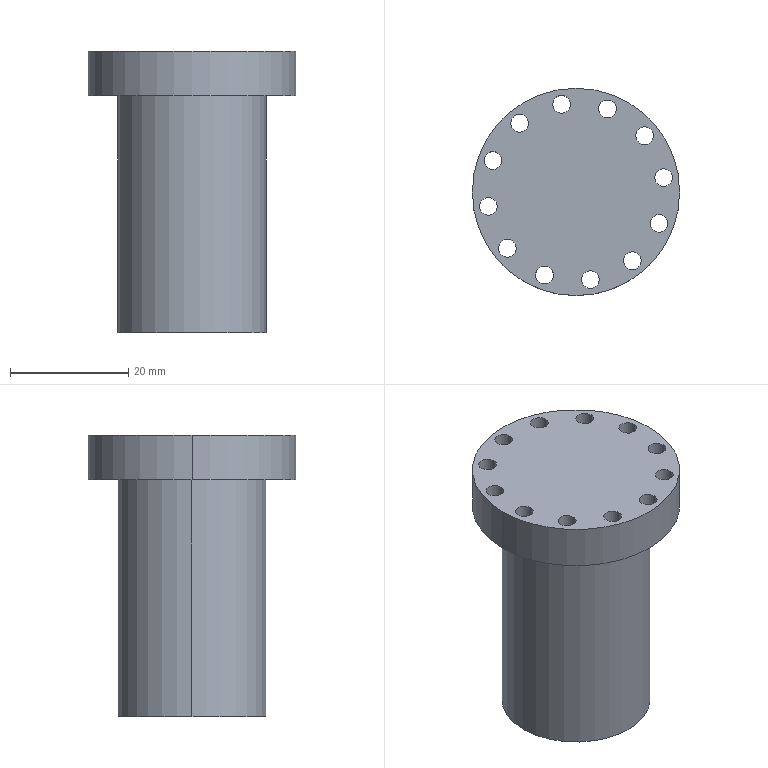Part | SolidWorks | features Cut 1, Extrusion 1, ICE 1 | 1 solid | 31 faces | box 35 x 35 x 47.5 mm | volume 26215 mm3 | cylinder 28 | plane 3 | commonest cylinder face diameters 3 x24 25 x2 35 x2
STEP:
#1=CARTESIAN_POINT('',(-76.803,10.969,0.));
#2=VERTEX_POINT('',#1);
#3=CARTESIAN_POINT('',(-73.803,10.969,0.));
#4=VERTEX_POINT('',#3);
#5=CARTESIAN_POINT('',(-75.303,10.969,0.));
#6=DIRECTION('',(0.,0.,1.));
#7=DIRECTION('',(1.,0.,0.));
#8=AXIS2_PLACEMENT_3D('',#5,#6,#7);
#9=CIRCLE('',#8,1.5);
#10=EDGE_CURVE('',#2,#4,#9,.T.);
#11=ORIENTED_EDGE('',*,*,#10,.F.);
#12=CARTESIAN_POINT('',(-76.803,10.969,7.5));
#13=VERTEX_POINT('',#12);
#14=CARTESIAN_POINT('',(-76.803,10.969,-40.));
#15=DIRECTION('',(0.,0.,1.));
#16=VECTOR('',#15,1000.);
#17=LINE('',#14,#16);
#18=EDGE_CURVE('',#2,#13,#17,.T.);
#19=ORIENTED_EDGE('',*,*,#18,.T.);
#20=CARTESIAN_POINT('',(-73.803,10.969,7.5));
#21=VERTEX_POINT('',#20);
#22=CARTESIAN_POINT('',(-75.303,10.969,7.5));
#23=DIRECTION('',(0.,0.,1.));
#24=DIRECTION('',(1.,0.,0.));
#25=AXIS2_PLACEMENT_3D('',#22,#23,#24);
#26=CIRCLE('',#25,1.5);
#27=EDGE_CURVE('',#13,#21,#26,.T.);
#28=ORIENTED_EDGE('',*,*,#27,.T.);
#29=CARTESIAN_POINT('',(-73.803,10.969,-40.));
#30=DIRECTION('',(0.,0.,1.));
#31=VECTOR('',#30,1000.);
#32=LINE('',#29,#31);
#33=EDGE_CURVE('',#4,#21,#32,.T.);
#34=ORIENTED_EDGE('',*,*,#33,.F.);
#35=EDGE_LOOP('',(#11,#19,#28,#34));
#36=FACE_OUTER_BOUND('',#35,.T.);
#37=CARTESIAN_POINT('',(-75.303,10.969,-40.));
#38=DIRECTION('',(0.,0.,1.));
#39=DIRECTION('',(1.,0.,0.));
#40=AXIS2_PLACEMENT_3D('',#37,#38,#39);
#41=CYLINDRICAL_SURFACE('',#40,1.5);
#42=ADVANCED_FACE('',(#36),#41,.F.);
#43=CARTESIAN_POINT('',(-69.077,10.197,0.));
#44=VERTEX_POINT('',#43);
#45=CARTESIAN_POINT('',(-66.077,10.197,0.));
#46=VERTEX_POINT('',#45);
#47=CARTESIAN_POINT('',(-67.577,10.197,0.));
#48=DIRECTION('',(0.,0.,1.));
#49=DIRECTION('',(1.,0.,0.));
#50=AXIS2_PLACEMENT_3D('',#47,#48,#49);
#51=CIRCLE('',#50,1.5);
#52=EDGE_CURVE('',#44,#46,#51,.T.);
#53=ORIENTED_EDGE('',*,*,#52,.F.);
#54=CARTESIAN_POINT('',(-69.077,10.197,7.5));
#55=VERTEX_POINT('',#54);
#56=CARTESIAN_POINT('',(-69.077,10.197,-40.));
#57=DIRECTION('',(0.,0.,1.));
#58=VECTOR('',#57,1000.);
#59=LINE('',#56,#58);
#60=EDGE_CURVE('',#44,#55,#59,.T.);
#61=ORIENTED_EDGE('',*,*,#60,.T.);
#62=CARTESIAN_POINT('',(-66.077,10.197,7.5));
#63=VERTEX_POINT('',#62);
#64=CARTESIAN_POINT('',(-67.577,10.197,7.5));
#65=DIRECTION('',(0.,0.,1.));
#66=DIRECTION('',(1.,0.,0.));
#67=AXIS2_PLACEMENT_3D('',#64,#65,#66);
#68=CIRCLE('',#67,1.5);
#69=EDGE_CURVE('',#55,#63,#68,.T.);
#70=ORIENTED_EDGE('',*,*,#69,.T.);
#71=CARTESIAN_POINT('',(-66.077,10.197,-40.));
#72=DIRECTION('',(0.,0.,1.));
#73=VECTOR('',#72,1000.);
#74=LINE('',#71,#73);
#75=EDGE_CURVE('',#46,#63,#74,.T.);
#76=ORIENTED_EDGE('',*,*,#75,.F.);
#77=EDGE_LOOP('',(#53,#61,#70,#76));
#78=FACE_OUTER_BOUND('',#77,.T.);
#79=CARTESIAN_POINT('',(-67.577,10.197,-40.));
#80=DIRECTION('',(0.,0.,1.));
#81=DIRECTION('',(1.,0.,0.));
#82=AXIS2_PLACEMENT_3D('',#79,#80,#81);
#83=CYLINDRICAL_SURFACE('',#82,1.5);
#84=ADVANCED_FACE('',(#78),#83,.F.);
#85=CARTESIAN_POINT('',(-62.,13.392,0.));
#86=VERTEX_POINT('',#85);
#87=CARTESIAN_POINT('',(-59.,13.392,0.));
#88=VERTEX_POINT('',#87);
#89=CARTESIAN_POINT('',(-60.5,13.392,0.));
#90=DIRECTION('',(0.,0.,1.));
#91=DIRECTION('',(1.,0.,0.));
#92=AXIS2_PLACEMENT_3D('',#89,#90,#91);
#93=CIRCLE('',#92,1.5);
#94=EDGE_CURVE('',#86,#88,#93,.T.);
#95=ORIENTED_EDGE('',*,*,#94,.F.);
#96=CARTESIAN_POINT('',(-62.,13.392,7.5));
#97=VERTEX_POINT('',#96);
#98=CARTESIAN_POINT('',(-62.,13.392,-40.));
#99=DIRECTION('',(0.,0.,1.));
#100=VECTOR('',#99,1000.);
#101=LINE('',#98,#100);
#102=EDGE_CURVE('',#86,#97,#101,.T.);
#103=ORIENTED_EDGE('',*,*,#102,.T.);
#104=CARTESIAN_POINT('',(-59.,13.392,7.5));
#105=VERTEX_POINT('',#104);
#106=CARTESIAN_POINT('',(-60.5,13.392,7.5));
#107=DIRECTION('',(0.,0.,1.));
#108=DIRECTION('',(1.,0.,0.));
#109=AXIS2_PLACEMENT_3D('',#106,#107,#108);
#110=CIRCLE('',#109,1.5);
#111=EDGE_CURVE('',#97,#105,#110,.T.);
#112=ORIENTED_EDGE('',*,*,#111,.T.);
#113=CARTESIAN_POINT('',(-59.,13.392,-40.));
#114=DIRECTION('',(0.,0.,1.));
#115=VECTOR('',#114,1000.);
#116=LINE('',#113,#115);
#117=EDGE_CURVE('',#88,#105,#116,.T.);
#118=ORIENTED_EDGE('',*,*,#117,.F.);
#119=EDGE_LOOP('',(#95,#103,#112,#118));
#120=FACE_OUTER_BOUND('',#119,.T.);
#121=CARTESIAN_POINT('',(-60.5,13.392,-40.));
#122=DIRECTION('',(0.,0.,1.));
#123=DIRECTION('',(1.,0.,0.));
#124=AXIS2_PLACEMENT_3D('',#121,#122,#123);
#125=CYLINDRICAL_SURFACE('',#124,1.5);
#126=ADVANCED_FACE('',(#120),#125,.F.);
#127=CARTESIAN_POINT('',(-57.469,19.697,0.));
#128=VERTEX_POINT('',#127);
#129=CARTESIAN_POINT('',(-54.469,19.697,0.));
#130=VERTEX_POINT('',#129);
#131=CARTESIAN_POINT('',(-55.969,19.697,0.));
#132=DIRECTION('',(0.,0.,1.));
#133=DIRECTION('',(1.,0.,0.));
#134=AXIS2_PLACEMENT_3D('',#131,#132,#133);
#135=CIRCLE('',#134,1.5);
#136=EDGE_CURVE('',#128,#130,#135,.T.);
#137=ORIENTED_EDGE('',*,*,#136,.F.);
#138=CARTESIAN_POINT('',(-57.469,19.697,7.5));
#139=VERTEX_POINT('',#138);
#140=CARTESIAN_POINT('',(-57.469,19.697,-40.));
#141=DIRECTION('',(0.,0.,1.));
#142=VECTOR('',#141,1000.);
#143=LINE('',#140,#142);
#144=EDGE_CURVE('',#128,#139,#143,.T.);
#145=ORIENTED_EDGE('',*,*,#144,.T.);
#146=CARTESIAN_POINT('',(-54.469,19.697,7.5));
#147=VERTEX_POINT('',#146);
#148=CARTESIAN_POINT('',(-55.969,19.697,7.5));
#149=DIRECTION('',(0.,0.,1.));
#150=DIRECTION('',(1.,0.,0.));
#151=AXIS2_PLACEMENT_3D('',#148,#149,#150);
#152=CIRCLE('',#151,1.5);
#153=EDGE_CURVE('',#139,#147,#152,.T.);
#154=ORIENTED_EDGE('',*,*,#153,.T.);
#155=CARTESIAN_POINT('',(-54.469,19.697,-40.));
#156=DIRECTION('',(0.,0.,1.));
#157=VECTOR('',#156,1000.);
#158=LINE('',#155,#157);
#159=EDGE_CURVE('',#130,#147,#158,.T.);
#160=ORIENTED_EDGE('',*,*,#159,.F.);
#161=EDGE_LOOP('',(#137,#145,#154,#160));
#162=FACE_OUTER_BOUND('',#161,.T.);
#163=CARTESIAN_POINT('',(-55.969,19.697,-40.));
#164=DIRECTION('',(0.,0.,1.));
#165=DIRECTION('',(1.,0.,0.));
#166=AXIS2_PLACEMENT_3D('',#163,#164,#165);
#167=CYLINDRICAL_SURFACE('',#166,1.5);
#168=ADVANCED_FACE('',(#162),#167,.F.);
#169=CARTESIAN_POINT('',(-56.697,27.423,0.));
#170=VERTEX_POINT('',#169);
#171=CARTESIAN_POINT('',(-53.697,27.423,0.));
#172=VERTEX_POINT('',#171);
#173=CARTESIAN_POINT('',(-55.197,27.423,0.));
#174=DIRECTION('',(0.,0.,1.));
#175=DIRECTION('',(1.,0.,0.));
#176=AXIS2_PLACEMENT_3D('',#173,#174,#175);
#177=CIRCLE('',#176,1.5);
#178=EDGE_CURVE('',#170,#172,#177,.T.);
#179=ORIENTED_EDGE('',*,*,#178,.F.);
#180=CARTESIAN_POINT('',(-56.697,27.423,7.5));
#181=VERTEX_POINT('',#180);
#182=CARTESIAN_POINT('',(-56.697,27.423,-40.));
#183=DIRECTION('',(0.,0.,1.));
#184=VECTOR('',#183,1000.);
#185=LINE('',#182,#184);
#186=EDGE_CURVE('',#170,#181,#185,.T.);
#187=ORIENTED_EDGE('',*,*,#186,.T.);
#188=CARTESIAN_POINT('',(-53.697,27.423,7.5));
#189=VERTEX_POINT('',#188);
#190=CARTESIAN_POINT('',(-55.197,27.423,7.5));
#191=DIRECTION('',(0.,0.,1.));
#192=DIRECTION('',(1.,0.,0.));
#193=AXIS2_PLACEMENT_3D('',#190,#191,#192);
#194=CIRCLE('',#193,1.5);
#195=EDGE_CURVE('',#181,#189,#194,.T.);
#196=ORIENTED_EDGE('',*,*,#195,.T.);
#197=CARTESIAN_POINT('',(-53.697,27.423,-40.));
#198=DIRECTION('',(0.,0.,1.));
#199=VECTOR('',#198,1000.);
#200=LINE('',#197,#199);
#201=EDGE_CURVE('',#172,#189,#200,.T.);
#202=ORIENTED_EDGE('',*,*,#201,.F.);
#203=EDGE_LOOP('',(#179,#187,#196,#202));
#204=FACE_OUTER_BOUND('',#203,.T.);
#205=CARTESIAN_POINT('',(-55.197,27.423,-40.));
#206=DIRECTION('',(0.,0.,1.));
#207=DIRECTION('',(1.,0.,0.));
#208=AXIS2_PLACEMENT_3D('',#205,#206,#207);
#209=CYLINDRICAL_SURFACE('',#208,1.5);
#210=ADVANCED_FACE('',(#204),#209,.F.);
#211=CARTESIAN_POINT('',(-59.892,34.5,0.));
#212=VERTEX_POINT('',#211);
#213=CARTESIAN_POINT('',(-56.892,34.5,0.));
#214=VERTEX_POINT('',#213);
#215=CARTESIAN_POINT('',(-58.392,34.5,0.));
#216=DIRECTION('',(0.,0.,1.));
#217=DIRECTION('',(1.,0.,0.));
#218=AXIS2_PLACEMENT_3D('',#215,#216,#217);
#219=CIRCLE('',#218,1.5);
#220=EDGE_CURVE('',#212,#214,#219,.T.);
#221=ORIENTED_EDGE('',*,*,#220,.F.);
#222=CARTESIAN_POINT('',(-59.892,34.5,7.5));
#223=VERTEX_POINT('',#222);
#224=CARTESIAN_POINT('',(-59.892,34.5,-40.));
#225=DIRECTION('',(0.,0.,1.));
#226=VECTOR('',#225,1000.);
#227=LINE('',#224,#226);
#228=EDGE_CURVE('',#212,#223,#227,.T.);
#229=ORIENTED_EDGE('',*,*,#228,.T.);
#230=CARTESIAN_POINT('',(-56.892,34.5,7.5));
#231=VERTEX_POINT('',#230);
#232=CARTESIAN_POINT('',(-58.392,34.5,7.5));
#233=DIRECTION('',(0.,0.,1.));
#234=DIRECTION('',(1.,0.,0.));
#235=AXIS2_PLACEMENT_3D('',#232,#233,#234);
#236=CIRCLE('',#235,1.5);
#237=EDGE_CURVE('',#223,#231,#236,.T.);
#238=ORIENTED_EDGE('',*,*,#237,.T.);
#239=CARTESIAN_POINT('',(-56.892,34.5,-40.));
#240=DIRECTION('',(0.,0.,1.));
#241=VECTOR('',#240,1000.);
#242=LINE('',#239,#241);
#243=EDGE_CURVE('',#214,#231,#242,.T.);
#244=ORIENTED_EDGE('',*,*,#243,.F.);
#245=EDGE_LOOP('',(#221,#229,#238,#244));
#246=FACE_OUTER_BOUND('',#245,.T.);
#247=CARTESIAN_POINT('',(-58.392,34.5,-40.));
#248=DIRECTION('',(0.,0.,1.));
#249=DIRECTION('',(1.,0.,0.));
#250=AXIS2_PLACEMENT_3D('',#247,#248,#249);
#251=CYLINDRICAL_SURFACE('',#250,1.5);
#252=ADVANCED_FACE('',(#246),#251,.F.);
#253=CARTESIAN_POINT('',(-66.197,39.031,0.));
#254=VERTEX_POINT('',#253);
#255=CARTESIAN_POINT('',(-63.197,39.031,0.));
#256=VERTEX_POINT('',#255);
#257=CARTESIAN_POINT('',(-64.697,39.031,0.));
#258=DIRECTION('',(0.,0.,1.));
#259=DIRECTION('',(1.,0.,0.));
#260=AXIS2_PLACEMENT_3D('',#257,#258,#259);
#261=CIRCLE('',#260,1.5);
#262=EDGE_CURVE('',#254,#256,#261,.T.);
#263=ORIENTED_EDGE('',*,*,#262,.F.);
#264=CARTESIAN_POINT('',(-66.197,39.031,7.5));
#265=VERTEX_POINT('',#264);
#266=CARTESIAN_POINT('',(-66.197,39.031,-40.));
#267=DIRECTION('',(0.,0.,1.));
#268=VECTOR('',#267,1000.);
#269=LINE('',#266,#268);
#270=EDGE_CURVE('',#254,#265,#269,.T.);
#271=ORIENTED_EDGE('',*,*,#270,.T.);
#272=CARTESIAN_POINT('',(-63.197,39.031,7.5));
#273=VERTEX_POINT('',#272);
#274=CARTESIAN_POINT('',(-64.697,39.031,7.5));
#275=DIRECTION('',(0.,0.,1.));
#276=DIRECTION('',(1.,0.,0.));
#277=AXIS2_PLACEMENT_3D('',#274,#275,#276);
#278=CIRCLE('',#277,1.5);
#279=EDGE_CURVE('',#265,#273,#278,.T.);
#280=ORIENTED_EDGE('',*,*,#279,.T.);
#281=CARTESIAN_POINT('',(-63.197,39.031,-40.));
#282=DIRECTION('',(0.,0.,1.));
#283=VECTOR('',#282,1000.);
#284=LINE('',#281,#283);
#285=EDGE_CURVE('',#256,#273,#284,.T.);
#286=ORIENTED_EDGE('',*,*,#285,.F.);
#287=EDGE_LOOP('',(#263,#271,#280,#286));
#288=FACE_OUTER_BOUND('',#287,.T.);
#289=CARTESIAN_POINT('',(-64.697,39.031,-40.));
#290=DIRECTION('',(0.,0.,1.));
#291=DIRECTION('',(1.,0.,0.));
#292=AXIS2_PLACEMENT_3D('',#289,#290,#291);
#293=CYLINDRICAL_SURFACE('',#292,1.5);
#294=ADVANCED_FACE('',(#288),#293,.F.);
#295=CARTESIAN_POINT('',(-73.923,39.803,0.));
#296=VERTEX_POINT('',#295);
#297=CARTESIAN_POINT('',(-70.923,39.803,0.));
#298=VERTEX_POINT('',#297);
#299=CARTESIAN_POINT('',(-72.423,39.803,0.));
#300=DIRECTION('',(0.,0.,1.));
#301=DIRECTION('',(1.,0.,0.));
#302=AXIS2_PLACEMENT_3D('',#299,#300,#301);
#303=CIRCLE('',#302,1.5);
#304=EDGE_CURVE('',#296,#298,#303,.T.);
#305=ORIENTED_EDGE('',*,*,#304,.F.);
#306=CARTESIAN_POINT('',(-73.923,39.803,7.5));
#307=VERTEX_POINT('',#306);
#308=CARTESIAN_POINT('',(-73.923,39.803,-40.));
#309=DIRECTION('',(0.,0.,1.));
#310=VECTOR('',#309,1000.);
#311=LINE('',#308,#310);
#312=EDGE_CURVE('',#296,#307,#311,.T.);
#313=ORIENTED_EDGE('',*,*,#312,.T.);
#314=CARTESIAN_POINT('',(-70.923,39.803,7.5));
#315=VERTEX_POINT('',#314);
#316=CARTESIAN_POINT('',(-72.423,39.803,7.5));
#317=DIRECTION('',(0.,0.,1.));
#318=DIRECTION('',(1.,0.,0.));
#319=AXIS2_PLACEMENT_3D('',#316,#317,#318);
#320=CIRCLE('',#319,1.5);
#321=EDGE_CURVE('',#307,#315,#320,.T.);
#322=ORIENTED_EDGE('',*,*,#321,.T.);
#323=CARTESIAN_POINT('',(-70.923,39.803,-40.));
#324=DIRECTION('',(0.,0.,1.));
#325=VECTOR('',#324,1000.);
#326=LINE('',#323,#325);
#327=EDGE_CURVE('',#298,#315,#326,.T.);
#328=ORIENTED_EDGE('',*,*,#327,.F.);
#329=EDGE_LOOP('',(#305,#313,#322,#328));
#330=FACE_OUTER_BOUND('',#329,.T.);
#331=CARTESIAN_POINT('',(-72.423,39.803,-40.));
#332=DIRECTION('',(0.,0.,1.));
#333=DIRECTION('',(1.,0.,0.));
#334=AXIS2_PLACEMENT_3D('',#331,#332,#333);
#335=CYLINDRICAL_SURFACE('',#334,1.5);
#336=ADVANCED_FACE('',(#330),#335,.F.);
#337=CARTESIAN_POINT('',(-81.,36.608,0.));
#338=VERTEX_POINT('',#337);
#339=CARTESIAN_POINT('',(-78.,36.608,0.));
#340=VERTEX_POINT('',#339);
#341=CARTESIAN_POINT('',(-79.5,36.608,0.));
#342=DIRECTION('',(0.,0.,1.));
#343=DIRECTION('',(1.,0.,0.));
#344=AXIS2_PLACEMENT_3D('',#341,#342,#343);
#345=CIRCLE('',#344,1.5);
#346=EDGE_CURVE('',#338,#340,#345,.T.);
#347=ORIENTED_EDGE('',*,*,#346,.F.);
#348=CARTESIAN_POINT('',(-81.,36.608,7.5));
#349=VERTEX_POINT('',#348);
#350=CARTESIAN_POINT('',(-81.,36.608,-40.));
#351=DIRECTION('',(0.,0.,1.));
#352=VECTOR('',#351,1000.);
#353=LINE('',#350,#352);
#354=EDGE_CURVE('',#338,#349,#353,.T.);
#355=ORIENTED_EDGE('',*,*,#354,.T.);
#356=CARTESIAN_POINT('',(-78.,36.608,7.5));
#357=VERTEX_POINT('',#356);
#358=CARTESIAN_POINT('',(-79.5,36.608,7.5));
#359=DIRECTION('',(0.,0.,1.));
#360=DIRECTION('',(1.,0.,0.));
#361=AXIS2_PLACEMENT_3D('',#358,#359,#360);
#362=CIRCLE('',#361,1.5);
#363=EDGE_CURVE('',#349,#357,#362,.T.);
#364=ORIENTED_EDGE('',*,*,#363,.T.);
#365=CARTESIAN_POINT('',(-78.,36.608,-40.));
#366=DIRECTION('',(0.,0.,1.));
#367=VECTOR('',#366,1000.);
#368=LINE('',#365,#367);
#369=EDGE_CURVE('',#340,#357,#368,.T.);
#370=ORIENTED_EDGE('',*,*,#369,.F.);
#371=EDGE_LOOP('',(#347,#355,#364,#370));
#372=FACE_OUTER_BOUND('',#371,.T.);
#373=CARTESIAN_POINT('',(-79.5,36.608,-40.));
#374=DIRECTION('',(0.,0.,1.));
#375=DIRECTION('',(1.,0.,0.));
#376=AXIS2_PLACEMENT_3D('',#373,#374,#375);
#377=CYLINDRICAL_SURFACE('',#376,1.5);
#378=ADVANCED_FACE('',(#372),#377,.F.);
#379=CARTESIAN_POINT('',(-85.531,30.303,0.));
#380=VERTEX_POINT('',#379);
#381=CARTESIAN_POINT('',(-82.531,30.303,0.));
#382=VERTEX_POINT('',#381);
#383=CARTESIAN_POINT('',(-84.031,30.303,0.));
#384=DIRECTION('',(0.,0.,1.));
#385=DIRECTION('',(1.,0.,0.));
#386=AXIS2_PLACEMENT_3D('',#383,#384,#385);
#387=CIRCLE('',#386,1.5);
#388=EDGE_CURVE('',#380,#382,#387,.T.);
#389=ORIENTED_EDGE('',*,*,#388,.F.);
#390=CARTESIAN_POINT('',(-85.531,30.303,7.5));
#391=VERTEX_POINT('',#390);
#392=CARTESIAN_POINT('',(-85.531,30.303,-40.));
#393=DIRECTION('',(0.,0.,1.));
#394=VECTOR('',#393,1000.);
#395=LINE('',#392,#394);
#396=EDGE_CURVE('',#380,#391,#395,.T.);
#397=ORIENTED_EDGE('',*,*,#396,.T.);
#398=CARTESIAN_POINT('',(-82.531,30.303,7.5));
#399=VERTEX_POINT('',#398);
#400=CARTESIAN_POINT('',(-84.031,30.303,7.5));
#401=DIRECTION('',(0.,0.,1.));
#402=DIRECTION('',(1.,0.,0.));
#403=AXIS2_PLACEMENT_3D('',#400,#401,#402);
#404=CIRCLE('',#403,1.5);
#405=EDGE_CURVE('',#391,#399,#404,.T.);
#406=ORIENTED_EDGE('',*,*,#405,.T.);
#407=CARTESIAN_POINT('',(-82.531,30.303,-40.));
#408=DIRECTION('',(0.,0.,1.));
#409=VECTOR('',#408,1000.);
#410=LINE('',#407,#409);
#411=EDGE_CURVE('',#382,#399,#410,.T.);
#412=ORIENTED_EDGE('',*,*,#411,.F.);
#413=EDGE_LOOP('',(#389,#397,#406,#412));
#414=FACE_OUTER_BOUND('',#413,.T.);
#415=CARTESIAN_POINT('',(-84.031,30.303,-40.));
#416=DIRECTION('',(0.,0.,1.));
#417=DIRECTION('',(1.,0.,0.));
#418=AXIS2_PLACEMENT_3D('',#415,#416,#417);
#419=CYLINDRICAL_SURFACE('',#418,1.5);
#420=ADVANCED_FACE('',(#414),#419,.F.);
#421=CARTESIAN_POINT('',(-86.303,22.577,0.));
#422=VERTEX_POINT('',#421);
#423=CARTESIAN_POINT('',(-83.303,22.577,0.));
#424=VERTEX_POINT('',#423);
#425=CARTESIAN_POINT('',(-84.803,22.577,0.));
#426=DIRECTION('',(0.,0.,1.));
#427=DIRECTION('',(1.,0.,0.));
#428=AXIS2_PLACEMENT_3D('',#425,#426,#427);
#429=CIRCLE('',#428,1.5);
#430=EDGE_CURVE('',#422,#424,#429,.T.);
#431=ORIENTED_EDGE('',*,*,#430,.F.);
#432=CARTESIAN_POINT('',(-86.303,22.577,7.5));
#433=VERTEX_POINT('',#432);
#434=CARTESIAN_POINT('',(-86.303,22.577,-40.));
#435=DIRECTION('',(0.,0.,1.));
#436=VECTOR('',#435,1000.);
#437=LINE('',#434,#436);
#438=EDGE_CURVE('',#422,#433,#437,.T.);
#439=ORIENTED_EDGE('',*,*,#438,.T.);
#440=CARTESIAN_POINT('',(-83.303,22.577,7.5));
#441=VERTEX_POINT('',#440);
#442=CARTESIAN_POINT('',(-84.803,22.577,7.5));
#443=DIRECTION('',(0.,0.,1.));
#444=DIRECTION('',(1.,0.,0.));
#445=AXIS2_PLACEMENT_3D('',#442,#443,#444);
#446=CIRCLE('',#445,1.5);
#447=EDGE_CURVE('',#433,#441,#446,.T.);
#448=ORIENTED_EDGE('',*,*,#447,.T.);
#449=CARTESIAN_POINT('',(-83.303,22.577,-40.));
#450=DIRECTION('',(0.,0.,1.));
#451=VECTOR('',#450,1000.);
#452=LINE('',#449,#451);
#453=EDGE_CURVE('',#424,#441,#452,.T.);
#454=ORIENTED_EDGE('',*,*,#453,.F.);
#455=EDGE_LOOP('',(#431,#439,#448,#454));
#456=FACE_OUTER_BOUND('',#455,.T.);
#457=CARTESIAN_POINT('',(-84.803,22.577,-40.));
#458=DIRECTION('',(0.,0.,1.));
#459=DIRECTION('',(1.,0.,0.));
#460=AXIS2_PLACEMENT_3D('',#457,#458,#459);
#461=CYLINDRICAL_SURFACE('',#460,1.5);
#462=ADVANCED_FACE('',(#456),#461,.F.);
#463=CARTESIAN_POINT('',(-83.108,15.5,0.));
#464=VERTEX_POINT('',#463);
#465=CARTESIAN_POINT('',(-80.108,15.5,0.));
#466=VERTEX_POINT('',#465);
#467=CARTESIAN_POINT('',(-81.608,15.5,0.));
#468=DIRECTION('',(0.,0.,1.));
#469=DIRECTION('',(1.,0.,0.));
#470=AXIS2_PLACEMENT_3D('',#467,#468,#469);
#471=CIRCLE('',#470,1.5);
#472=EDGE_CURVE('',#464,#466,#471,.T.);
#473=ORIENTED_EDGE('',*,*,#472,.F.);
#474=CARTESIAN_POINT('',(-83.108,15.5,7.5));
#475=VERTEX_POINT('',#474);
#476=CARTESIAN_POINT('',(-83.108,15.5,-40.));
#477=DIRECTION('',(0.,0.,1.));
#478=VECTOR('',#477,1000.);
#479=LINE('',#476,#478);
#480=EDGE_CURVE('',#464,#475,#479,.T.);
#481=ORIENTED_EDGE('',*,*,#480,.T.);
#482=CARTESIAN_POINT('',(-80.108,15.5,7.5));
#483=VERTEX_POINT('',#482);
#484=CARTESIAN_POINT('',(-81.608,15.5,7.5));
#485=DIRECTION('',(0.,0.,1.));
#486=DIRECTION('',(1.,0.,0.));
#487=AXIS2_PLACEMENT_3D('',#484,#485,#486);
#488=CIRCLE('',#487,1.5);
#489=EDGE_CURVE('',#475,#483,#488,.T.);
#490=ORIENTED_EDGE('',*,*,#489,.T.);
#491=CARTESIAN_POINT('',(-80.108,15.5,-40.));
#492=DIRECTION('',(0.,0.,1.));
#493=VECTOR('',#492,1000.);
#494=LINE('',#491,#493);
#495=EDGE_CURVE('',#466,#483,#494,.T.);
#496=ORIENTED_EDGE('',*,*,#495,.F.);
#497=EDGE_LOOP('',(#473,#481,#490,#496));
#498=FACE_OUTER_BOUND('',#497,.T.);
#499=CARTESIAN_POINT('',(-81.608,15.5,-40.));
#500=DIRECTION('',(0.,0.,1.));
#501=DIRECTION('',(1.,0.,0.));
#502=AXIS2_PLACEMENT_3D('',#499,#500,#501);
#503=CYLINDRICAL_SURFACE('',#502,1.5);
#504=ADVANCED_FACE('',(#498),#503,.F.);
#505=CARTESIAN_POINT('',(-82.5,25.,-40.));
#506=VERTEX_POINT('',#505);
#507=CARTESIAN_POINT('',(-57.5,25.,-40.));
#508=VERTEX_POINT('',#507);
#509=CARTESIAN_POINT('',(-70.,25.,-40.));
#510=DIRECTION('',(0.,0.,-1.));
#511=DIRECTION('',(-1.,0.,0.));
#512=AXIS2_PLACEMENT_3D('',#509,#510,#511);
#513=CIRCLE('',#512,12.5);
#514=EDGE_CURVE('',#506,#508,#513,.T.);
#515=ORIENTED_EDGE('',*,*,#514,.F.);
#516=CARTESIAN_POINT('',(-82.5,25.,0.));
#517=VERTEX_POINT('',#516);
#518=CARTESIAN_POINT('',(-82.5,25.,-40.));
#519=DIRECTION('',(0.,0.,1.));
#520=VECTOR('',#519,1000.);
#521=LINE('',#518,#520);
#522=EDGE_CURVE('',#506,#517,#521,.T.);
#523=ORIENTED_EDGE('',*,*,#522,.T.);
#524=CARTESIAN_POINT('',(-57.5,25.,0.));
#525=VERTEX_POINT('',#524);
#526=CARTESIAN_POINT('',(-70.,25.,0.));
#527=DIRECTION('',(0.,0.,-1.));
#528=DIRECTION('',(-1.,0.,0.));
#529=AXIS2_PLACEMENT_3D('',#526,#527,#528);
#530=CIRCLE('',#529,12.5);
#531=EDGE_CURVE('',#517,#525,#530,.T.);
#532=ORIENTED_EDGE('',*,*,#531,.T.);
#533=CARTESIAN_POINT('',(-57.5,25.,-40.));
#534=DIRECTION('',(0.,0.,1.));
#535=VECTOR('',#534,1000.);
#536=LINE('',#533,#535);
#537=EDGE_CURVE('',#508,#525,#536,.T.);
#538=ORIENTED_EDGE('',*,*,#537,.F.);
#539=EDGE_LOOP('',(#515,#523,#532,#538));
#540=FACE_OUTER_BOUND('',#539,.T.);
#541=CARTESIAN_POINT('',(-70.,25.,-40.));
#542=DIRECTION('',(0.,0.,1.));
#543=DIRECTION('',(1.,0.,0.));
#544=AXIS2_PLACEMENT_3D('',#541,#542,#543);
#545=CYLINDRICAL_SURFACE('',#544,12.5);
#546=ADVANCED_FACE('',(#540),#545,.T.);
#547=CARTESIAN_POINT('',(-52.5,25.,7.5));
#548=VERTEX_POINT('',#547);
#549=CARTESIAN_POINT('',(-87.5,25.,7.5));
#550=VERTEX_POINT('',#549);
#551=CARTESIAN_POINT('',(-70.,25.,7.5));
#552=DIRECTION('',(0.,0.,1.));
#553=DIRECTION('',(1.,0.,0.));
#554=AXIS2_PLACEMENT_3D('',#551,#552,#553);
#555=CIRCLE('',#554,17.5);
#556=EDGE_CURVE('',#548,#550,#555,.T.);
#557=ORIENTED_EDGE('',*,*,#556,.F.);
#558=CARTESIAN_POINT('',(-52.5,25.,0.));
#559=VERTEX_POINT('',#558);
#560=CARTESIAN_POINT('',(-52.5,25.,7.5));
#561=DIRECTION('',(0.,0.,-1.));
#562=VECTOR('',#561,1000.);
#563=LINE('',#560,#562);
#564=EDGE_CURVE('',#548,#559,#563,.T.);
#565=ORIENTED_EDGE('',*,*,#564,.T.);
#566=CARTESIAN_POINT('',(-87.5,25.,0.));
#567=VERTEX_POINT('',#566);
#568=CARTESIAN_POINT('',(-70.,25.,0.));
#569=DIRECTION('',(0.,0.,1.));
#570=DIRECTION('',(1.,0.,0.));
#571=AXIS2_PLACEMENT_3D('',#568,#569,#570);
#572=CIRCLE('',#571,17.5);
#573=EDGE_CURVE('',#559,#567,#572,.T.);
#574=ORIENTED_EDGE('',*,*,#573,.T.);
#575=CARTESIAN_POINT('',(-87.5,25.,7.5));
#576=DIRECTION('',(0.,0.,-1.));
#577=VECTOR('',#576,1000.);
#578=LINE('',#575,#577);
#579=EDGE_CURVE('',#550,#567,#578,.T.);
#580=ORIENTED_EDGE('',*,*,#579,.F.);
#581=EDGE_LOOP('',(#557,#565,#574,#580));
#582=FACE_OUTER_BOUND('',#581,.T.);
#583=CARTESIAN_POINT('',(-70.,25.,7.5));
#584=DIRECTION('',(0.,0.,-1.));
#585=DIRECTION('',(-1.,0.,0.));
#586=AXIS2_PLACEMENT_3D('',#583,#584,#585);
#587=CYLINDRICAL_SURFACE('',#586,17.5);
#588=ADVANCED_FACE('',(#582),#587,.T.);
#589=ORIENTED_EDGE('',*,*,#564,.F.);
#590=CARTESIAN_POINT('',(-70.,25.,7.5));
#591=DIRECTION('',(0.,0.,1.));
#592=DIRECTION('',(1.,0.,0.));
#593=AXIS2_PLACEMENT_3D('',#590,#591,#592);
#594=CIRCLE('',#593,17.5);
#595=EDGE_CURVE('',#550,#548,#594,.T.);
#596=ORIENTED_EDGE('',*,*,#595,.F.);
#597=ORIENTED_EDGE('',*,*,#579,.T.);
#598=CARTESIAN_POINT('',(-70.,25.,0.));
#599=DIRECTION('',(0.,0.,1.));
#600=DIRECTION('',(1.,0.,0.));
#601=AXIS2_PLACEMENT_3D('',#598,#599,#600);
#602=CIRCLE('',#601,17.5);
#603=EDGE_CURVE('',#567,#559,#602,.T.);
#604=ORIENTED_EDGE('',*,*,#603,.T.);
#605=EDGE_LOOP('',(#589,#596,#597,#604));
#606=FACE_OUTER_BOUND('',#605,.T.);
#607=CARTESIAN_POINT('',(-70.,25.,7.5));
#608=DIRECTION('',(0.,0.,-1.));
#609=DIRECTION('',(-1.,0.,0.));
#610=AXIS2_PLACEMENT_3D('',#607,#608,#609);
#611=CYLINDRICAL_SURFACE('',#610,17.5);
#612=ADVANCED_FACE('',(#606),#611,.T.);
#613=CARTESIAN_POINT('',(-75.303,10.969,7.5));
#614=DIRECTION('',(0.,0.,1.));
#615=DIRECTION('',(1.,0.,0.));
#616=AXIS2_PLACEMENT_3D('',#613,#614,#615);
#617=CIRCLE('',#616,1.5);
#618=EDGE_CURVE('',#21,#13,#617,.T.);
#619=ORIENTED_EDGE('',*,*,#618,.F.);
#620=ORIENTED_EDGE('',*,*,#27,.F.);
#621=EDGE_LOOP('',(#619,#620));
#622=FACE_BOUND('',#621,.T.);
#623=CARTESIAN_POINT('',(-67.577,10.197,7.5));
#624=DIRECTION('',(0.,0.,1.));
#625=DIRECTION('',(1.,0.,0.));
#626=AXIS2_PLACEMENT_3D('',#623,#624,#625);
#627=CIRCLE('',#626,1.5);
#628=EDGE_CURVE('',#63,#55,#627,.T.);
#629=ORIENTED_EDGE('',*,*,#628,.F.);
#630=ORIENTED_EDGE('',*,*,#69,.F.);
#631=EDGE_LOOP('',(#629,#630));
#632=FACE_BOUND('',#631,.T.);
#633=CARTESIAN_POINT('',(-60.5,13.392,7.5));
#634=DIRECTION('',(0.,0.,1.));
#635=DIRECTION('',(1.,0.,0.));
#636=AXIS2_PLACEMENT_3D('',#633,#634,#635);
#637=CIRCLE('',#636,1.5);
#638=EDGE_CURVE('',#105,#97,#637,.T.);
#639=ORIENTED_EDGE('',*,*,#638,.F.);
#640=ORIENTED_EDGE('',*,*,#111,.F.);
#641=EDGE_LOOP('',(#639,#640));
#642=FACE_BOUND('',#641,.T.);
#643=CARTESIAN_POINT('',(-55.969,19.697,7.5));
#644=DIRECTION('',(0.,0.,1.));
#645=DIRECTION('',(1.,0.,0.));
#646=AXIS2_PLACEMENT_3D('',#643,#644,#645);
#647=CIRCLE('',#646,1.5);
#648=EDGE_CURVE('',#147,#139,#647,.T.);
#649=ORIENTED_EDGE('',*,*,#648,.F.);
#650=ORIENTED_EDGE('',*,*,#153,.F.);
#651=EDGE_LOOP('',(#649,#650));
#652=FACE_BOUND('',#651,.T.);
#653=CARTESIAN_POINT('',(-55.197,27.423,7.5));
#654=DIRECTION('',(0.,0.,1.));
#655=DIRECTION('',(1.,0.,0.));
#656=AXIS2_PLACEMENT_3D('',#653,#654,#655);
#657=CIRCLE('',#656,1.5);
#658=EDGE_CURVE('',#189,#181,#657,.T.);
#659=ORIENTED_EDGE('',*,*,#658,.F.);
#660=ORIENTED_EDGE('',*,*,#195,.F.);
#661=EDGE_LOOP('',(#659,#660));
#662=FACE_BOUND('',#661,.T.);
#663=CARTESIAN_POINT('',(-58.392,34.5,7.5));
#664=DIRECTION('',(0.,0.,1.));
#665=DIRECTION('',(1.,0.,0.));
#666=AXIS2_PLACEMENT_3D('',#663,#664,#665);
#667=CIRCLE('',#666,1.5);
#668=EDGE_CURVE('',#231,#223,#667,.T.);
#669=ORIENTED_EDGE('',*,*,#668,.F.);
#670=ORIENTED_EDGE('',*,*,#237,.F.);
#671=EDGE_LOOP('',(#669,#670));
#672=FACE_BOUND('',#671,.T.);
#673=CARTESIAN_POINT('',(-64.697,39.031,7.5));
#674=DIRECTION('',(0.,0.,1.));
#675=DIRECTION('',(1.,0.,0.));
#676=AXIS2_PLACEMENT_3D('',#673,#674,#675);
#677=CIRCLE('',#676,1.5);
#678=EDGE_CURVE('',#273,#265,#677,.T.);
#679=ORIENTED_EDGE('',*,*,#678,.F.);
#680=ORIENTED_EDGE('',*,*,#279,.F.);
#681=EDGE_LOOP('',(#679,#680));
#682=FACE_BOUND('',#681,.T.);
#683=CARTESIAN_POINT('',(-72.423,39.803,7.5));
#684=DIRECTION('',(0.,0.,1.));
#685=DIRECTION('',(1.,0.,0.));
#686=AXIS2_PLACEMENT_3D('',#683,#684,#685);
#687=CIRCLE('',#686,1.5);
#688=EDGE_CURVE('',#315,#307,#687,.T.);
#689=ORIENTED_EDGE('',*,*,#688,.F.);
#690=ORIENTED_EDGE('',*,*,#321,.F.);
#691=EDGE_LOOP('',(#689,#690));
#692=FACE_BOUND('',#691,.T.);
#693=CARTESIAN_POINT('',(-79.5,36.608,7.5));
#694=DIRECTION('',(0.,0.,1.));
#695=DIRECTION('',(1.,0.,0.));
#696=AXIS2_PLACEMENT_3D('',#693,#694,#695);
#697=CIRCLE('',#696,1.5);
#698=EDGE_CURVE('',#357,#349,#697,.T.);
#699=ORIENTED_EDGE('',*,*,#698,.F.);
#700=ORIENTED_EDGE('',*,*,#363,.F.);
#701=EDGE_LOOP('',(#699,#700));
#702=FACE_BOUND('',#701,.T.);
#703=CARTESIAN_POINT('',(-84.031,30.303,7.5));
#704=DIRECTION('',(0.,0.,1.));
#705=DIRECTION('',(1.,0.,0.));
#706=AXIS2_PLACEMENT_3D('',#703,#704,#705);
#707=CIRCLE('',#706,1.5);
#708=EDGE_CURVE('',#399,#391,#707,.T.);
#709=ORIENTED_EDGE('',*,*,#708,.F.);
#710=ORIENTED_EDGE('',*,*,#405,.F.);
#711=EDGE_LOOP('',(#709,#710));
#712=FACE_BOUND('',#711,.T.);
#713=CARTESIAN_POINT('',(-84.803,22.577,7.5));
#714=DIRECTION('',(0.,0.,1.));
#715=DIRECTION('',(1.,0.,0.));
#716=AXIS2_PLACEMENT_3D('',#713,#714,#715);
#717=CIRCLE('',#716,1.5);
#718=EDGE_CURVE('',#441,#433,#717,.T.);
#719=ORIENTED_EDGE('',*,*,#718,.F.);
#720=ORIENTED_EDGE('',*,*,#447,.F.);
#721=EDGE_LOOP('',(#719,#720));
#722=FACE_BOUND('',#721,.T.);
#723=CARTESIAN_POINT('',(-81.608,15.5,7.5));
#724=DIRECTION('',(0.,0.,1.));
#725=DIRECTION('',(1.,0.,0.));
#726=AXIS2_PLACEMENT_3D('',#723,#724,#725);
#727=CIRCLE('',#726,1.5);
#728=EDGE_CURVE('',#483,#475,#727,.T.);
#729=ORIENTED_EDGE('',*,*,#728,.F.);
#730=ORIENTED_EDGE('',*,*,#489,.F.);
#731=EDGE_LOOP('',(#729,#730));
#732=FACE_BOUND('',#731,.T.);
#733=ORIENTED_EDGE('',*,*,#595,.T.);
#734=ORIENTED_EDGE('',*,*,#556,.T.);
#735=EDGE_LOOP('',(#733,#734));
#736=FACE_OUTER_BOUND('',#735,.T.);
#737=CARTESIAN_POINT('',(-70.,25.,7.5));
#738=DIRECTION('',(0.,0.,1.));
#739=DIRECTION('',(1.,0.,0.));
#740=AXIS2_PLACEMENT_3D('',#737,#738,#739);
#741=PLANE('',#740);
#742=ADVANCED_FACE('',(#622,#632,#642,#652,#662,#672,#682,#692,#702,#712,#722,#732,#736),#741,.T.);
#743=CARTESIAN_POINT('',(-75.303,10.969,0.));
#744=DIRECTION('',(0.,0.,1.));
#745=DIRECTION('',(1.,0.,0.));
#746=AXIS2_PLACEMENT_3D('',#743,#744,#745);
#747=CIRCLE('',#746,1.5);
#748=EDGE_CURVE('',#4,#2,#747,.T.);
#749=ORIENTED_EDGE('',*,*,#748,.T.);
#750=ORIENTED_EDGE('',*,*,#10,.T.);
#751=EDGE_LOOP('',(#749,#750));
#752=FACE_BOUND('',#751,.T.);
#753=CARTESIAN_POINT('',(-67.577,10.197,0.));
#754=DIRECTION('',(0.,0.,1.));
#755=DIRECTION('',(1.,0.,0.));
#756=AXIS2_PLACEMENT_3D('',#753,#754,#755);
#757=CIRCLE('',#756,1.5);
#758=EDGE_CURVE('',#46,#44,#757,.T.);
#759=ORIENTED_EDGE('',*,*,#758,.T.);
#760=ORIENTED_EDGE('',*,*,#52,.T.);
#761=EDGE_LOOP('',(#759,#760));
#762=FACE_BOUND('',#761,.T.);
#763=CARTESIAN_POINT('',(-60.5,13.392,0.));
#764=DIRECTION('',(0.,0.,1.));
#765=DIRECTION('',(1.,0.,0.));
#766=AXIS2_PLACEMENT_3D('',#763,#764,#765);
#767=CIRCLE('',#766,1.5);
#768=EDGE_CURVE('',#88,#86,#767,.T.);
#769=ORIENTED_EDGE('',*,*,#768,.T.);
#770=ORIENTED_EDGE('',*,*,#94,.T.);
#771=EDGE_LOOP('',(#769,#770));
#772=FACE_BOUND('',#771,.T.);
#773=CARTESIAN_POINT('',(-55.969,19.697,0.));
#774=DIRECTION('',(0.,0.,1.));
#775=DIRECTION('',(1.,0.,0.));
#776=AXIS2_PLACEMENT_3D('',#773,#774,#775);
#777=CIRCLE('',#776,1.5);
#778=EDGE_CURVE('',#130,#128,#777,.T.);
#779=ORIENTED_EDGE('',*,*,#778,.T.);
#780=ORIENTED_EDGE('',*,*,#136,.T.);
#781=EDGE_LOOP('',(#779,#780));
#782=FACE_BOUND('',#781,.T.);
#783=CARTESIAN_POINT('',(-55.197,27.423,0.));
#784=DIRECTION('',(0.,0.,1.));
#785=DIRECTION('',(1.,0.,0.));
#786=AXIS2_PLACEMENT_3D('',#783,#784,#785);
#787=CIRCLE('',#786,1.5);
#788=EDGE_CURVE('',#172,#170,#787,.T.);
#789=ORIENTED_EDGE('',*,*,#788,.T.);
#790=ORIENTED_EDGE('',*,*,#178,.T.);
#791=EDGE_LOOP('',(#789,#790));
#792=FACE_BOUND('',#791,.T.);
#793=CARTESIAN_POINT('',(-58.392,34.5,0.));
#794=DIRECTION('',(0.,0.,1.));
#795=DIRECTION('',(1.,0.,0.));
#796=AXIS2_PLACEMENT_3D('',#793,#794,#795);
#797=CIRCLE('',#796,1.5);
#798=EDGE_CURVE('',#214,#212,#797,.T.);
#799=ORIENTED_EDGE('',*,*,#798,.T.);
#800=ORIENTED_EDGE('',*,*,#220,.T.);
#801=EDGE_LOOP('',(#799,#800));
#802=FACE_BOUND('',#801,.T.);
#803=CARTESIAN_POINT('',(-64.697,39.031,0.));
#804=DIRECTION('',(0.,0.,1.));
#805=DIRECTION('',(1.,0.,0.));
#806=AXIS2_PLACEMENT_3D('',#803,#804,#805);
#807=CIRCLE('',#806,1.5);
#808=EDGE_CURVE('',#256,#254,#807,.T.);
#809=ORIENTED_EDGE('',*,*,#808,.T.);
#810=ORIENTED_EDGE('',*,*,#262,.T.);
#811=EDGE_LOOP('',(#809,#810));
#812=FACE_BOUND('',#811,.T.);
#813=CARTESIAN_POINT('',(-72.423,39.803,0.));
#814=DIRECTION('',(0.,0.,1.));
#815=DIRECTION('',(1.,0.,0.));
#816=AXIS2_PLACEMENT_3D('',#813,#814,#815);
#817=CIRCLE('',#816,1.5);
#818=EDGE_CURVE('',#298,#296,#817,.T.);
#819=ORIENTED_EDGE('',*,*,#818,.T.);
#820=ORIENTED_EDGE('',*,*,#304,.T.);
#821=EDGE_LOOP('',(#819,#820));
#822=FACE_BOUND('',#821,.T.);
#823=CARTESIAN_POINT('',(-79.5,36.608,0.));
#824=DIRECTION('',(0.,0.,1.));
#825=DIRECTION('',(1.,0.,0.));
#826=AXIS2_PLACEMENT_3D('',#823,#824,#825);
#827=CIRCLE('',#826,1.5);
#828=EDGE_CURVE('',#340,#338,#827,.T.);
#829=ORIENTED_EDGE('',*,*,#828,.T.);
#830=ORIENTED_EDGE('',*,*,#346,.T.);
#831=EDGE_LOOP('',(#829,#830));
#832=FACE_BOUND('',#831,.T.);
#833=CARTESIAN_POINT('',(-84.031,30.303,0.));
#834=DIRECTION('',(0.,0.,1.));
#835=DIRECTION('',(1.,0.,0.));
#836=AXIS2_PLACEMENT_3D('',#833,#834,#835);
#837=CIRCLE('',#836,1.5);
#838=EDGE_CURVE('',#382,#380,#837,.T.);
#839=ORIENTED_EDGE('',*,*,#838,.T.);
#840=ORIENTED_EDGE('',*,*,#388,.T.);
#841=EDGE_LOOP('',(#839,#840));
#842=FACE_BOUND('',#841,.T.);
#843=CARTESIAN_POINT('',(-84.803,22.577,0.));
#844=DIRECTION('',(0.,0.,1.));
#845=DIRECTION('',(1.,0.,0.));
#846=AXIS2_PLACEMENT_3D('',#843,#844,#845);
#847=CIRCLE('',#846,1.5);
#848=EDGE_CURVE('',#424,#422,#847,.T.);
#849=ORIENTED_EDGE('',*,*,#848,.T.);
#850=ORIENTED_EDGE('',*,*,#430,.T.);
#851=EDGE_LOOP('',(#849,#850));
#852=FACE_BOUND('',#851,.T.);
#853=CARTESIAN_POINT('',(-81.608,15.5,0.));
#854=DIRECTION('',(0.,0.,1.));
#855=DIRECTION('',(1.,0.,0.));
#856=AXIS2_PLACEMENT_3D('',#853,#854,#855);
#857=CIRCLE('',#856,1.5);
#858=EDGE_CURVE('',#466,#464,#857,.T.);
#859=ORIENTED_EDGE('',*,*,#858,.T.);
#860=ORIENTED_EDGE('',*,*,#472,.T.);
#861=EDGE_LOOP('',(#859,#860));
#862=FACE_BOUND('',#861,.T.);
#863=CARTESIAN_POINT('',(-70.,25.,0.));
#864=DIRECTION('',(0.,0.,-1.));
#865=DIRECTION('',(-1.,0.,0.));
#866=AXIS2_PLACEMENT_3D('',#863,#864,#865);
#867=CIRCLE('',#866,12.5);
#868=EDGE_CURVE('',#525,#517,#867,.T.);
#869=ORIENTED_EDGE('',*,*,#868,.F.);
#870=ORIENTED_EDGE('',*,*,#531,.F.);
#871=EDGE_LOOP('',(#869,#870));
#872=FACE_BOUND('',#871,.T.);
#873=ORIENTED_EDGE('',*,*,#603,.F.);
#874=ORIENTED_EDGE('',*,*,#573,.F.);
#875=EDGE_LOOP('',(#873,#874));
#876=FACE_OUTER_BOUND('',#875,.T.);
#877=CARTESIAN_POINT('',(-70.,25.,0.));
#878=DIRECTION('',(0.,0.,1.));
#879=DIRECTION('',(1.,0.,0.));
#880=AXIS2_PLACEMENT_3D('',#877,#878,#879);
#881=PLANE('',#880);
#882=ADVANCED_FACE('',(#752,#762,#772,#782,#792,#802,#812,#822,#832,#842,#852,#862,#872,#876),#881,.F.);
#883=ORIENTED_EDGE('',*,*,#522,.F.);
#884=CARTESIAN_POINT('',(-70.,25.,-40.));
#885=DIRECTION('',(0.,0.,-1.));
#886=DIRECTION('',(-1.,0.,0.));
#887=AXIS2_PLACEMENT_3D('',#884,#885,#886);
#888=CIRCLE('',#887,12.5);
#889=EDGE_CURVE('',#508,#506,#888,.T.);
#890=ORIENTED_EDGE('',*,*,#889,.F.);
#891=ORIENTED_EDGE('',*,*,#537,.T.);
#892=ORIENTED_EDGE('',*,*,#868,.T.);
#893=EDGE_LOOP('',(#883,#890,#891,#892));
#894=FACE_OUTER_BOUND('',#893,.T.);
#895=CARTESIAN_POINT('',(-70.,25.,-40.));
#896=DIRECTION('',(0.,0.,1.));
#897=DIRECTION('',(1.,0.,0.));
#898=AXIS2_PLACEMENT_3D('',#895,#896,#897);
#899=CYLINDRICAL_SURFACE('',#898,12.5);
#900=ADVANCED_FACE('',(#894),#899,.T.);
#901=ORIENTED_EDGE('',*,*,#889,.T.);
#902=ORIENTED_EDGE('',*,*,#514,.T.);
#903=EDGE_LOOP('',(#901,#902));
#904=FACE_OUTER_BOUND('',#903,.T.);
#905=CARTESIAN_POINT('',(-70.,25.,-40.));
#906=DIRECTION('',(0.,0.,-1.));
#907=DIRECTION('',(-1.,0.,0.));
#908=AXIS2_PLACEMENT_3D('',#905,#906,#907);
#909=PLANE('',#908);
#910=ADVANCED_FACE('',(#904),#909,.T.);
#911=ORIENTED_EDGE('',*,*,#480,.F.);
#912=ORIENTED_EDGE('',*,*,#858,.F.);
#913=ORIENTED_EDGE('',*,*,#495,.T.);
#914=ORIENTED_EDGE('',*,*,#728,.T.);
#915=EDGE_LOOP('',(#911,#912,#913,#914));
#916=FACE_OUTER_BOUND('',#915,.T.);
#917=CARTESIAN_POINT('',(-81.608,15.5,-40.));
#918=DIRECTION('',(0.,0.,1.));
#919=DIRECTION('',(1.,0.,0.));
#920=AXIS2_PLACEMENT_3D('',#917,#918,#919);
#921=CYLINDRICAL_SURFACE('',#920,1.5);
#922=ADVANCED_FACE('',(#916),#921,.F.);
#923=ORIENTED_EDGE('',*,*,#438,.F.);
#924=ORIENTED_EDGE('',*,*,#848,.F.);
#925=ORIENTED_EDGE('',*,*,#453,.T.);
#926=ORIENTED_EDGE('',*,*,#718,.T.);
#927=EDGE_LOOP('',(#923,#924,#925,#926));
#928=FACE_OUTER_BOUND('',#927,.T.);
#929=CARTESIAN_POINT('',(-84.803,22.577,-40.));
#930=DIRECTION('',(0.,0.,1.));
#931=DIRECTION('',(1.,0.,0.));
#932=AXIS2_PLACEMENT_3D('',#929,#930,#931);
#933=CYLINDRICAL_SURFACE('',#932,1.5);
#934=ADVANCED_FACE('',(#928),#933,.F.);
#935=ORIENTED_EDGE('',*,*,#396,.F.);
#936=ORIENTED_EDGE('',*,*,#838,.F.);
#937=ORIENTED_EDGE('',*,*,#411,.T.);
#938=ORIENTED_EDGE('',*,*,#708,.T.);
#939=EDGE_LOOP('',(#935,#936,#937,#938));
#940=FACE_OUTER_BOUND('',#939,.T.);
#941=CARTESIAN_POINT('',(-84.031,30.303,-40.));
#942=DIRECTION('',(0.,0.,1.));
#943=DIRECTION('',(1.,0.,0.));
#944=AXIS2_PLACEMENT_3D('',#941,#942,#943);
#945=CYLINDRICAL_SURFACE('',#944,1.5);
#946=ADVANCED_FACE('',(#940),#945,.F.);
#947=ORIENTED_EDGE('',*,*,#354,.F.);
#948=ORIENTED_EDGE('',*,*,#828,.F.);
#949=ORIENTED_EDGE('',*,*,#369,.T.);
#950=ORIENTED_EDGE('',*,*,#698,.T.);
#951=EDGE_LOOP('',(#947,#948,#949,#950));
#952=FACE_OUTER_BOUND('',#951,.T.);
#953=CARTESIAN_POINT('',(-79.5,36.608,-40.));
#954=DIRECTION('',(0.,0.,1.));
#955=DIRECTION('',(1.,0.,0.));
#956=AXIS2_PLACEMENT_3D('',#953,#954,#955);
#957=CYLINDRICAL_SURFACE('',#956,1.5);
#958=ADVANCED_FACE('',(#952),#957,.F.);
#959=ORIENTED_EDGE('',*,*,#312,.F.);
#960=ORIENTED_EDGE('',*,*,#818,.F.);
#961=ORIENTED_EDGE('',*,*,#327,.T.);
#962=ORIENTED_EDGE('',*,*,#688,.T.);
#963=EDGE_LOOP('',(#959,#960,#961,#962));
#964=FACE_OUTER_BOUND('',#963,.T.);
#965=CARTESIAN_POINT('',(-72.423,39.803,-40.));
#966=DIRECTION('',(0.,0.,1.));
#967=DIRECTION('',(1.,0.,0.));
#968=AXIS2_PLACEMENT_3D('',#965,#966,#967);
#969=CYLINDRICAL_SURFACE('',#968,1.5);
#970=ADVANCED_FACE('',(#964),#969,.F.);
#971=ORIENTED_EDGE('',*,*,#270,.F.);
#972=ORIENTED_EDGE('',*,*,#808,.F.);
#973=ORIENTED_EDGE('',*,*,#285,.T.);
#974=ORIENTED_EDGE('',*,*,#678,.T.);
#975=EDGE_LOOP('',(#971,#972,#973,#974));
#976=FACE_OUTER_BOUND('',#975,.T.);
#977=CARTESIAN_POINT('',(-64.697,39.031,-40.));
#978=DIRECTION('',(0.,0.,1.));
#979=DIRECTION('',(1.,0.,0.));
#980=AXIS2_PLACEMENT_3D('',#977,#978,#979);
#981=CYLINDRICAL_SURFACE('',#980,1.5);
#982=ADVANCED_FACE('',(#976),#981,.F.);
#983=ORIENTED_EDGE('',*,*,#228,.F.);
#984=ORIENTED_EDGE('',*,*,#798,.F.);
#985=ORIENTED_EDGE('',*,*,#243,.T.);
#986=ORIENTED_EDGE('',*,*,#668,.T.);
#987=EDGE_LOOP('',(#983,#984,#985,#986));
#988=FACE_OUTER_BOUND('',#987,.T.);
#989=CARTESIAN_POINT('',(-58.392,34.5,-40.));
#990=DIRECTION('',(0.,0.,1.));
#991=DIRECTION('',(1.,0.,0.));
#992=AXIS2_PLACEMENT_3D('',#989,#990,#991);
#993=CYLINDRICAL_SURFACE('',#992,1.5);
#994=ADVANCED_FACE('',(#988),#993,.F.);
#995=ORIENTED_EDGE('',*,*,#186,.F.);
#996=ORIENTED_EDGE('',*,*,#788,.F.);
#997=ORIENTED_EDGE('',*,*,#201,.T.);
#998=ORIENTED_EDGE('',*,*,#658,.T.);
#999=EDGE_LOOP('',(#995,#996,#997,#998));
#1000=FACE_OUTER_BOUND('',#999,.T.);
#1001=CARTESIAN_POINT('',(-55.197,27.423,-40.));
#1002=DIRECTION('',(0.,0.,1.));
#1003=DIRECTION('',(1.,0.,0.));
#1004=AXIS2_PLACEMENT_3D('',#1001,#1002,#1003);
#1005=CYLINDRICAL_SURFACE('',#1004,1.5);
#1006=ADVANCED_FACE('',(#1000),#1005,.F.);
#1007=ORIENTED_EDGE('',*,*,#144,.F.);
#1008=ORIENTED_EDGE('',*,*,#778,.F.);
#1009=ORIENTED_EDGE('',*,*,#159,.T.);
#1010=ORIENTED_EDGE('',*,*,#648,.T.);
#1011=EDGE_LOOP('',(#1007,#1008,#1009,#1010));
#1012=FACE_OUTER_BOUND('',#1011,.T.);
#1013=CARTESIAN_POINT('',(-55.969,19.697,-40.));
#1014=DIRECTION('',(0.,0.,1.));
#1015=DIRECTION('',(1.,0.,0.));
#1016=AXIS2_PLACEMENT_3D('',#1013,#1014,#1015);
#1017=CYLINDRICAL_SURFACE('',#1016,1.5);
#1018=ADVANCED_FACE('',(#1012),#1017,.F.);
#1019=ORIENTED_EDGE('',*,*,#102,.F.);
#1020=ORIENTED_EDGE('',*,*,#768,.F.);
#1021=ORIENTED_EDGE('',*,*,#117,.T.);
#1022=ORIENTED_EDGE('',*,*,#638,.T.);
#1023=EDGE_LOOP('',(#1019,#1020,#1021,#1022));
#1024=FACE_OUTER_BOUND('',#1023,.T.);
#1025=CARTESIAN_POINT('',(-60.5,13.392,-40.));
#1026=DIRECTION('',(0.,0.,1.));
#1027=DIRECTION('',(1.,0.,0.));
#1028=AXIS2_PLACEMENT_3D('',#1025,#1026,#1027);
#1029=CYLINDRICAL_SURFACE('',#1028,1.5);
#1030=ADVANCED_FACE('',(#1024),#1029,.F.);
#1031=ORIENTED_EDGE('',*,*,#60,.F.);
#1032=ORIENTED_EDGE('',*,*,#758,.F.);
#1033=ORIENTED_EDGE('',*,*,#75,.T.);
#1034=ORIENTED_EDGE('',*,*,#628,.T.);
#1035=EDGE_LOOP('',(#1031,#1032,#1033,#1034));
#1036=FACE_OUTER_BOUND('',#1035,.T.);
#1037=CARTESIAN_POINT('',(-67.577,10.197,-40.));
#1038=DIRECTION('',(0.,0.,1.));
#1039=DIRECTION('',(1.,0.,0.));
#1040=AXIS2_PLACEMENT_3D('',#1037,#1038,#1039);
#1041=CYLINDRICAL_SURFACE('',#1040,1.5);
#1042=ADVANCED_FACE('',(#1036),#1041,.F.);
#1043=ORIENTED_EDGE('',*,*,#18,.F.);
#1044=ORIENTED_EDGE('',*,*,#748,.F.);
#1045=ORIENTED_EDGE('',*,*,#33,.T.);
#1046=ORIENTED_EDGE('',*,*,#618,.T.);
#1047=EDGE_LOOP('',(#1043,#1044,#1045,#1046));
#1048=FACE_OUTER_BOUND('',#1047,.T.);
#1049=CARTESIAN_POINT('',(-75.303,10.969,-40.));
#1050=DIRECTION('',(0.,0.,1.));
#1051=DIRECTION('',(1.,0.,0.));
#1052=AXIS2_PLACEMENT_3D('',#1049,#1050,#1051);
#1053=CYLINDRICAL_SURFACE('',#1052,1.5);
#1054=ADVANCED_FACE('',(#1048),#1053,.F.);
#1055=CLOSED_SHELL('',(#42,#84,#126,#168,#210,#252,#294,#336,#378,#420,#462,#504,#546,#588,#612,#742,#882,#900,#910,#922,#934,#946,#958,#970,#982,#994,#1006,#1018,#1030,#1042,#1054));
#1056=MANIFOLD_SOLID_BREP('',#1055);
#1057=CARTESIAN_POINT('',(0.,0.,0.));
#1058=DIRECTION('',(0.,0.,1.));
#1059=DIRECTION('',(1.,0.,0.));
#1060=AXIS2_PLACEMENT_3D('',#1057,#1058,#1059);
#1061=(LENGTH_UNIT()NAMED_UNIT(*)SI_UNIT(.MILLI.,.METRE.));
#1062=UNCERTAINTY_MEASURE_WITH_UNIT(LENGTH_MEASURE(0.00001),#1061,'','');
#1063=(NAMED_UNIT(*)PLANE_ANGLE_UNIT()SI_UNIT($,.RADIAN.));
#1064=(NAMED_UNIT(*)SI_UNIT($,.STERADIAN.)SOLID_ANGLE_UNIT());
#1065=(GEOMETRIC_REPRESENTATION_CONTEXT(3)GLOBAL_UNCERTAINTY_ASSIGNED_CONTEXT((#1062))GLOBAL_UNIT_ASSIGNED_CONTEXT((#1061,#1063,#1064))REPRESENTATION_CONTEXT('',''));
#1066=ADVANCED_BREP_SHAPE_REPRESENTATION('',(#1056,#1060),#1065);